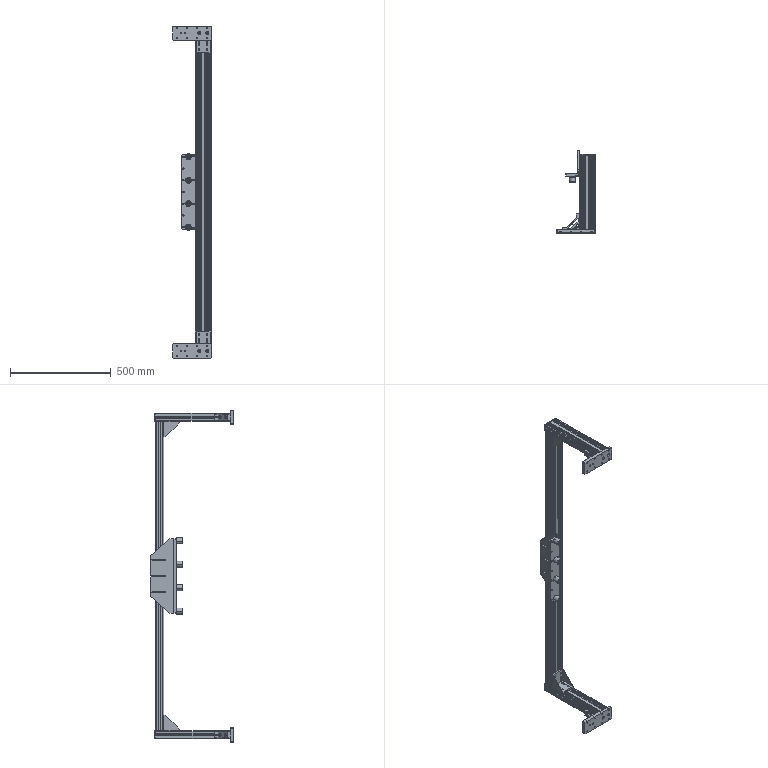Part | SolidWorks | features ReferencePattern 6, DerivedHolePattern 1, MirrorCompFeat 1 | 21 solids | 1309 faces | box 190 x 410 x 1645 mm | volume 3631798 mm3 | plane 792 | cylinder 445 | spline 64 | cone 8 | commonest cylinder face diameters 9 x63 8.5 x48 8 x40 6.6 x38 6.8 x34 11 x32